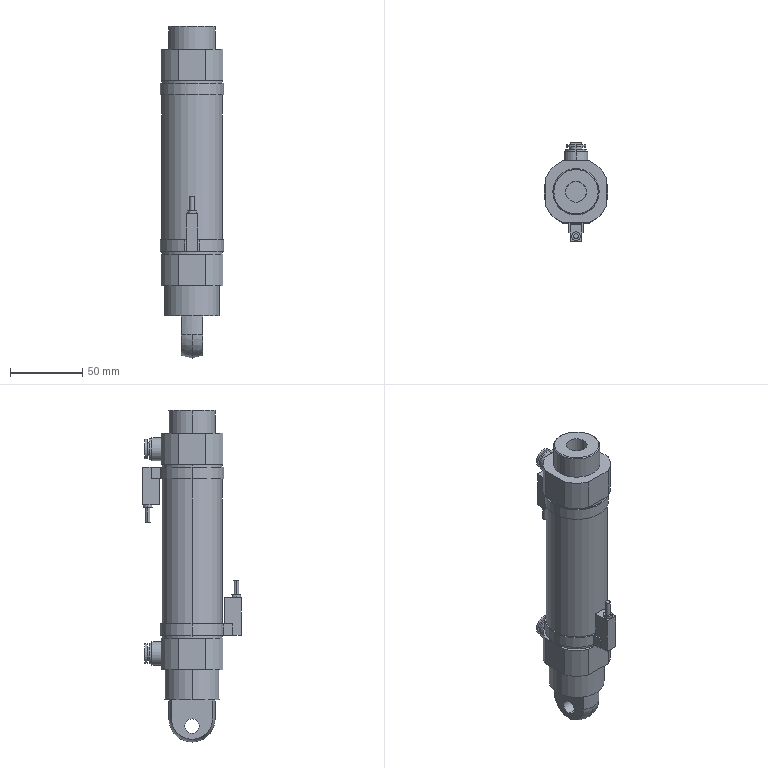Part | STEP file | body_A_CDM2C40F_75_C76_0_ | 3 solids | 145 faces | box 44 x 68 x 229 mm | volume 272575 mm3 | cylinder 74 | plane 63 | cone 6 | sphere 2 | commonest cylinder face diameters 44 x8 46.5 x8 13.36 x6 42 x6 3.4 x4 6 x4